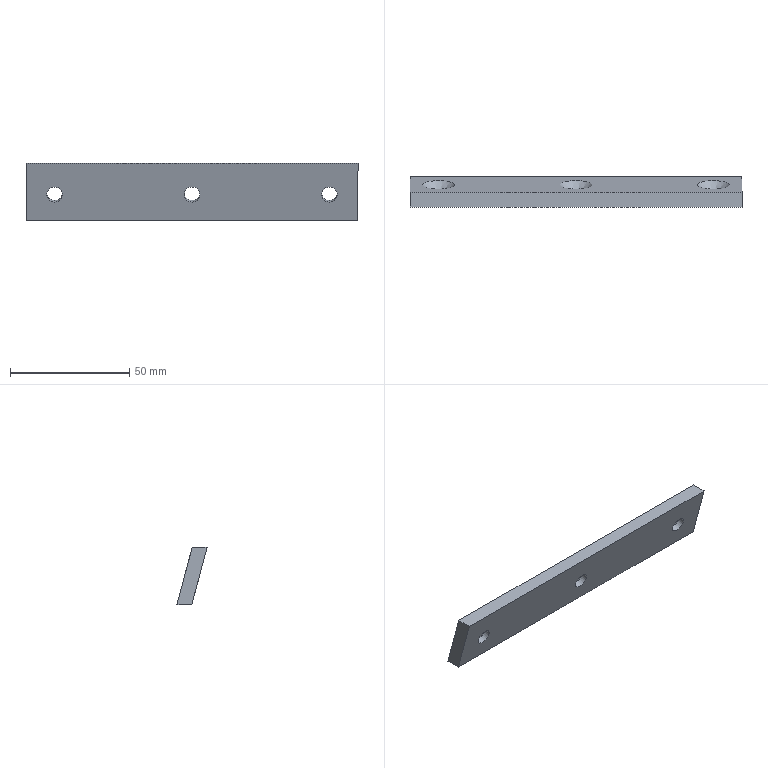Part | STEP file | solid 16 | 1 solid | 12 faces | box 139 x 12.642 x 24 mm | volume 19581 mm3 | plane 6 | cone 3 | cylinder 3 | commonest cylinder face diameters 6.5 x3